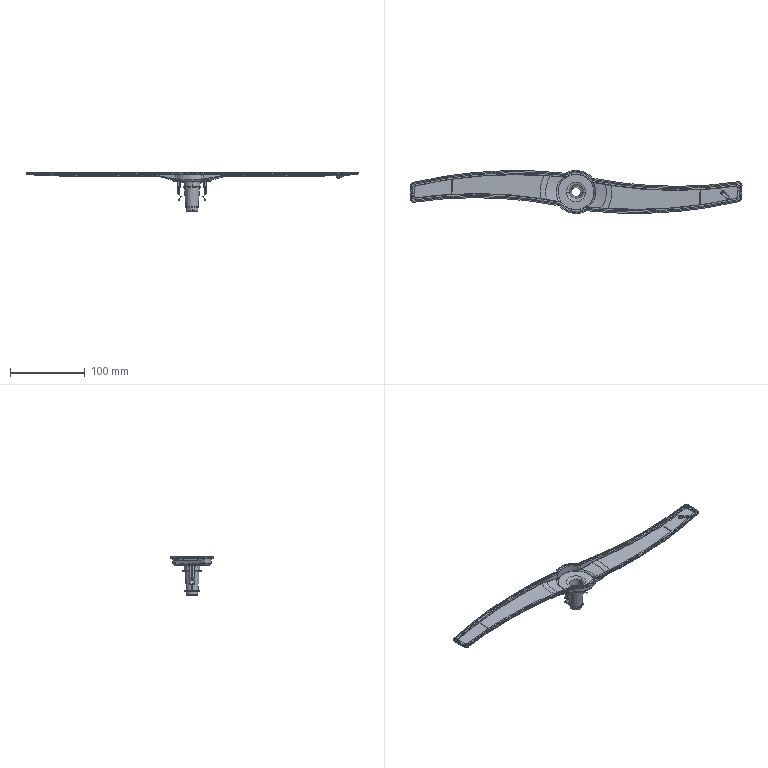Part | STEP file | ZXW722-L-16 | 1 solid | 589 faces | box 443.493 x 58 x 51.016 mm | volume 34498 mm3 | spline 194 | cylinder 194 | torus 82 | plane 73 | cone 24 | sphere 22 | commonest cylinder face diameters 0.6 x79 1 x20 6 x8 9 x8 10 x8 2 x7